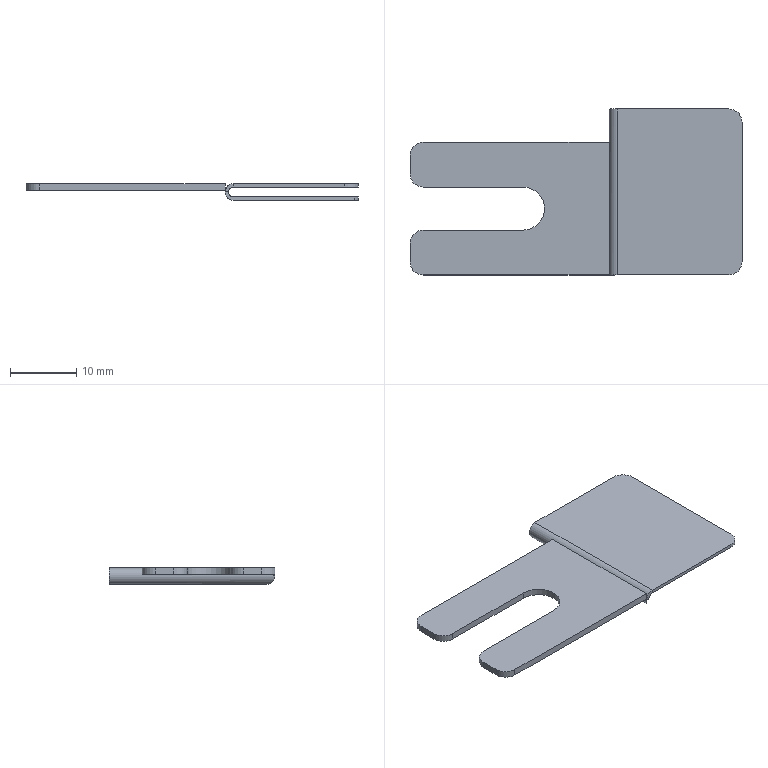Part | SolidWorks | features ICE 4, Fillet 2, FlatPattern 2, SMBaseFlange 2, SheetMetal 2, MirrorSolid 1 | 2 solids | 33 faces | box 50 x 25 x 2.5 mm | volume 876.083 mm3 | plane 22 | cylinder 11 | commonest cylinder face diameters 4 x8 1.5 x1 2.5 x1 6.5 x1
STEP:
#1=CARTESIAN_POINT('',(1.25,0.,0.));
#2=VERTEX_POINT('',#1);
#3=CARTESIAN_POINT('',(0.,0.,-1.25));
#4=VERTEX_POINT('',#3);
#5=CARTESIAN_POINT('',(1.25,0.,-1.25));
#6=DIRECTION('',(0.,-1.,0.));
#7=DIRECTION('',(0.,0.,1.));
#8=AXIS2_PLACEMENT_3D('',#5,#6,#7);
#9=CIRCLE('',#8,1.25);
#10=EDGE_CURVE('',#2,#4,#9,.T.);
#11=ORIENTED_EDGE('',*,*,#10,.T.);
#12=CARTESIAN_POINT('',(0.5,0.,-1.25));
#13=VERTEX_POINT('',#12);
#14=CARTESIAN_POINT('',(20.,0.,-1.25));
#15=DIRECTION('',(-1.,0.,0.));
#16=VECTOR('',#15,1000.);
#17=LINE('',#14,#16);
#18=EDGE_CURVE('',#13,#4,#17,.T.);
#19=ORIENTED_EDGE('',*,*,#18,.F.);
#20=CARTESIAN_POINT('',(1.25,0.,-0.5));
#21=VERTEX_POINT('',#20);
#22=CARTESIAN_POINT('',(1.25,0.,-1.25));
#23=DIRECTION('',(0.,-1.,0.));
#24=DIRECTION('',(1.,0.,0.));
#25=AXIS2_PLACEMENT_3D('',#22,#23,#24);
#26=CIRCLE('',#25,0.75);
#27=EDGE_CURVE('',#21,#13,#26,.T.);
#28=ORIENTED_EDGE('',*,*,#27,.F.);
#29=CARTESIAN_POINT('',(1.25,0.,0.));
#30=DIRECTION('',(0.,0.,-1.));
#31=VECTOR('',#30,1000.);
#32=LINE('',#29,#31);
#33=EDGE_CURVE('',#2,#21,#32,.T.);
#34=ORIENTED_EDGE('',*,*,#33,.F.);
#35=EDGE_LOOP('',(#11,#19,#28,#34));
#36=FACE_OUTER_BOUND('',#35,.T.);
#37=CARTESIAN_POINT('',(1.25,0.,0.));
#38=DIRECTION('',(0.,-1.,0.));
#39=DIRECTION('',(0.,0.,-1.));
#40=AXIS2_PLACEMENT_3D('',#37,#38,#39);
#41=PLANE('',#40);
#42=ADVANCED_FACE('',(#36),#41,.T.);
#43=CARTESIAN_POINT('',(1.25,25.,-2.5));
#44=VERTEX_POINT('',#43);
#45=CARTESIAN_POINT('',(1.25,25.,-2.));
#46=VERTEX_POINT('',#45);
#47=CARTESIAN_POINT('',(1.25,25.,-2.5));
#48=DIRECTION('',(0.,0.,1.));
#49=VECTOR('',#48,1000.);
#50=LINE('',#47,#49);
#51=EDGE_CURVE('',#44,#46,#50,.T.);
#52=ORIENTED_EDGE('',*,*,#51,.F.);
#53=CARTESIAN_POINT('',(1.25,25.,0.));
#54=VERTEX_POINT('',#53);
#55=CARTESIAN_POINT('',(1.25,25.,-1.25));
#56=DIRECTION('',(0.,-1.,0.));
#57=DIRECTION('',(0.,0.,1.));
#58=AXIS2_PLACEMENT_3D('',#55,#56,#57);
#59=CIRCLE('',#58,1.25);
#60=EDGE_CURVE('',#54,#44,#59,.T.);
#61=ORIENTED_EDGE('',*,*,#60,.F.);
#62=CARTESIAN_POINT('',(1.25,25.,-0.5));
#63=VERTEX_POINT('',#62);
#64=CARTESIAN_POINT('',(1.25,25.,-0.5));
#65=DIRECTION('',(0.,0.,1.));
#66=VECTOR('',#65,1000.);
#67=LINE('',#64,#66);
#68=EDGE_CURVE('',#63,#54,#67,.T.);
#69=ORIENTED_EDGE('',*,*,#68,.F.);
#70=CARTESIAN_POINT('',(1.25,25.,-1.25));
#71=DIRECTION('',(0.,-1.,0.));
#72=DIRECTION('',(1.,0.,0.));
#73=AXIS2_PLACEMENT_3D('',#70,#71,#72);
#74=CIRCLE('',#73,0.75);
#75=EDGE_CURVE('',#63,#46,#74,.T.);
#76=ORIENTED_EDGE('',*,*,#75,.T.);
#77=EDGE_LOOP('',(#52,#61,#69,#76));
#78=FACE_OUTER_BOUND('',#77,.T.);
#79=CARTESIAN_POINT('',(1.25,25.,-2.5));
#80=DIRECTION('',(0.,1.,0.));
#81=DIRECTION('',(0.,0.,1.));
#82=AXIS2_PLACEMENT_3D('',#79,#80,#81);
#83=PLANE('',#82);
#84=ADVANCED_FACE('',(#78),#83,.T.);
#85=CARTESIAN_POINT('',(18.,25.,-2.));
#86=VERTEX_POINT('',#85);
#87=CARTESIAN_POINT('',(1.25,25.,-2.));
#88=DIRECTION('',(1.,0.,0.));
#89=VECTOR('',#88,1000.);
#90=LINE('',#87,#89);
#91=EDGE_CURVE('',#46,#86,#90,.T.);
#92=ORIENTED_EDGE('',*,*,#91,.T.);
#93=CARTESIAN_POINT('',(18.,25.,-2.5));
#94=VERTEX_POINT('',#93);
#95=CARTESIAN_POINT('',(18.,25.,-0.5));
#96=DIRECTION('',(0.,0.,-1.));
#97=VECTOR('',#96,1000.);
#98=LINE('',#95,#97);
#99=EDGE_CURVE('',#86,#94,#98,.T.);
#100=ORIENTED_EDGE('',*,*,#99,.T.);
#101=CARTESIAN_POINT('',(1.25,25.,-2.5));
#102=DIRECTION('',(1.,0.,0.));
#103=VECTOR('',#102,1000.);
#104=LINE('',#101,#103);
#105=EDGE_CURVE('',#44,#94,#104,.T.);
#106=ORIENTED_EDGE('',*,*,#105,.F.);
#107=ORIENTED_EDGE('',*,*,#51,.T.);
#108=EDGE_LOOP('',(#92,#100,#106,#107));
#109=FACE_OUTER_BOUND('',#108,.T.);
#110=CARTESIAN_POINT('',(1.25,25.,-0.5));
#111=DIRECTION('',(0.,1.,0.));
#112=DIRECTION('',(0.,0.,1.));
#113=AXIS2_PLACEMENT_3D('',#110,#111,#112);
#114=PLANE('',#113);
#115=ADVANCED_FACE('',(#109),#114,.T.);
#116=CARTESIAN_POINT('',(18.,0.,-0.5));
#117=VERTEX_POINT('',#116);
#118=CARTESIAN_POINT('',(20.,0.,-0.5));
#119=DIRECTION('',(-1.,0.,0.));
#120=VECTOR('',#119,1000.);
#121=LINE('',#118,#120);
#122=EDGE_CURVE('',#117,#21,#121,.T.);
#123=ORIENTED_EDGE('',*,*,#122,.F.);
#124=CARTESIAN_POINT('',(18.,0.,0.));
#125=VERTEX_POINT('',#124);
#126=CARTESIAN_POINT('',(18.,0.,-2.));
#127=DIRECTION('',(0.,0.,1.));
#128=VECTOR('',#127,1000.);
#129=LINE('',#126,#128);
#130=EDGE_CURVE('',#117,#125,#129,.T.);
#131=ORIENTED_EDGE('',*,*,#130,.T.);
#132=CARTESIAN_POINT('',(20.,0.,0.));
#133=DIRECTION('',(-1.,0.,0.));
#134=VECTOR('',#133,1000.);
#135=LINE('',#132,#134);
#136=EDGE_CURVE('',#125,#2,#135,.T.);
#137=ORIENTED_EDGE('',*,*,#136,.T.);
#138=ORIENTED_EDGE('',*,*,#33,.T.);
#139=EDGE_LOOP('',(#123,#131,#137,#138));
#140=FACE_OUTER_BOUND('',#139,.T.);
#141=CARTESIAN_POINT('',(1.25,0.,-2.));
#142=DIRECTION('',(0.,-1.,0.));
#143=DIRECTION('',(0.,0.,-1.));
#144=AXIS2_PLACEMENT_3D('',#141,#142,#143);
#145=PLANE('',#144);
#146=ADVANCED_FACE('',(#140),#145,.T.);
#147=CARTESIAN_POINT('',(20.,23.,-2.));
#148=VERTEX_POINT('',#147);
#149=CARTESIAN_POINT('',(20.,20.828,-2.));
#150=VERTEX_POINT('',#149);
#151=CARTESIAN_POINT('',(20.,25.,-2.));
#152=DIRECTION('',(0.,-1.,0.));
#153=VECTOR('',#152,1000.);
#154=LINE('',#151,#153);
#155=EDGE_CURVE('',#148,#150,#154,.T.);
#156=ORIENTED_EDGE('',*,*,#155,.F.);
#157=CARTESIAN_POINT('',(18.,23.,-2.));
#158=DIRECTION('',(0.,0.,1.));
#159=DIRECTION('',(-1.,0.,0.));
#160=AXIS2_PLACEMENT_3D('',#157,#158,#159);
#161=CIRCLE('',#160,2.);
#162=EDGE_CURVE('',#148,#86,#161,.T.);
#163=ORIENTED_EDGE('',*,*,#162,.T.);
#164=ORIENTED_EDGE('',*,*,#91,.F.);
#165=CARTESIAN_POINT('',(1.25,1.25,-2.));
#166=VERTEX_POINT('',#165);
#167=CARTESIAN_POINT('',(1.25,25.,-2.));
#168=DIRECTION('',(0.,-1.,0.));
#169=VECTOR('',#168,1000.);
#170=LINE('',#167,#169);
#171=EDGE_CURVE('',#46,#166,#170,.T.);
#172=ORIENTED_EDGE('',*,*,#171,.T.);
#173=CARTESIAN_POINT('',(19.414,19.414,-2.));
#174=VERTEX_POINT('',#173);
#175=CARTESIAN_POINT('',(13.125,13.125,-2.));
#176=DIRECTION('',(0.7071,0.7071,0.));
#177=VECTOR('',#176,1000.);
#178=LINE('',#175,#177);
#179=EDGE_CURVE('',#166,#174,#178,.T.);
#180=ORIENTED_EDGE('',*,*,#179,.T.);
#181=CARTESIAN_POINT('',(18.,20.828,-2.));
#182=DIRECTION('',(0.,0.,1.));
#183=DIRECTION('',(-1.,0.,0.));
#184=AXIS2_PLACEMENT_3D('',#181,#182,#183);
#185=CIRCLE('',#184,2.);
#186=EDGE_CURVE('',#174,#150,#185,.T.);
#187=ORIENTED_EDGE('',*,*,#186,.T.);
#188=EDGE_LOOP('',(#156,#163,#164,#172,#180,#187));
#189=FACE_OUTER_BOUND('',#188,.T.);
#190=CARTESIAN_POINT('',(1.25,25.,-2.));
#191=DIRECTION('',(0.,0.,-1.));
#192=DIRECTION('',(-1.,0.,0.));
#193=AXIS2_PLACEMENT_3D('',#190,#191,#192);
#194=PLANE('',#193);
#195=ADVANCED_FACE('',(#189),#194,.F.);
#196=CARTESIAN_POINT('',(20.,23.,-2.5));
#197=VERTEX_POINT('',#196);
#198=CARTESIAN_POINT('',(20.,20.828,-2.5));
#199=VERTEX_POINT('',#198);
#200=CARTESIAN_POINT('',(20.,25.,-2.5));
#201=DIRECTION('',(0.,-1.,0.));
#202=VECTOR('',#201,1000.);
#203=LINE('',#200,#202);
#204=EDGE_CURVE('',#197,#199,#203,.T.);
#205=ORIENTED_EDGE('',*,*,#204,.F.);
#206=CARTESIAN_POINT('',(20.,23.,-2.5));
#207=DIRECTION('',(0.,0.,1.));
#208=VECTOR('',#207,1000.);
#209=LINE('',#206,#208);
#210=EDGE_CURVE('',#197,#148,#209,.T.);
#211=ORIENTED_EDGE('',*,*,#210,.T.);
#212=ORIENTED_EDGE('',*,*,#155,.T.);
#213=CARTESIAN_POINT('',(20.,20.828,-2.5));
#214=DIRECTION('',(0.,0.,-1.));
#215=VECTOR('',#214,1000.);
#216=LINE('',#213,#215);
#217=EDGE_CURVE('',#150,#199,#216,.T.);
#218=ORIENTED_EDGE('',*,*,#217,.T.);
#219=EDGE_LOOP('',(#205,#211,#212,#218));
#220=FACE_OUTER_BOUND('',#219,.T.);
#221=CARTESIAN_POINT('',(20.,25.,-2.5));
#222=DIRECTION('',(1.,0.,0.));
#223=DIRECTION('',(0.,0.,-1.));
#224=AXIS2_PLACEMENT_3D('',#221,#222,#223);
#225=PLANE('',#224);
#226=ADVANCED_FACE('',(#220),#225,.T.);
#227=ORIENTED_EDGE('',*,*,#105,.T.);
#228=CARTESIAN_POINT('',(18.,23.,-2.5));
#229=DIRECTION('',(0.,0.,-1.));
#230=DIRECTION('',(-1.,0.,0.));
#231=AXIS2_PLACEMENT_3D('',#228,#229,#230);
#232=CIRCLE('',#231,2.);
#233=EDGE_CURVE('',#94,#197,#232,.T.);
#234=ORIENTED_EDGE('',*,*,#233,.T.);
#235=ORIENTED_EDGE('',*,*,#204,.T.);
#236=CARTESIAN_POINT('',(19.414,19.414,-2.5));
#237=VERTEX_POINT('',#236);
#238=CARTESIAN_POINT('',(18.,20.828,-2.5));
#239=DIRECTION('',(0.,0.,-1.));
#240=DIRECTION('',(-1.,0.,0.));
#241=AXIS2_PLACEMENT_3D('',#238,#239,#240);
#242=CIRCLE('',#241,2.);
#243=EDGE_CURVE('',#199,#237,#242,.T.);
#244=ORIENTED_EDGE('',*,*,#243,.T.);
#245=CARTESIAN_POINT('',(1.25,1.25,-2.5));
#246=VERTEX_POINT('',#245);
#247=CARTESIAN_POINT('',(0.,0.,-2.5));
#248=DIRECTION('',(0.7071,0.7071,0.));
#249=VECTOR('',#248,1000.);
#250=LINE('',#247,#249);
#251=EDGE_CURVE('',#246,#237,#250,.T.);
#252=ORIENTED_EDGE('',*,*,#251,.F.);
#253=CARTESIAN_POINT('',(1.25,25.,-2.5));
#254=DIRECTION('',(0.,-1.,0.));
#255=VECTOR('',#254,1000.);
#256=LINE('',#253,#255);
#257=EDGE_CURVE('',#44,#246,#256,.T.);
#258=ORIENTED_EDGE('',*,*,#257,.F.);
#259=EDGE_LOOP('',(#227,#234,#235,#244,#252,#258));
#260=FACE_OUTER_BOUND('',#259,.T.);
#261=CARTESIAN_POINT('',(1.25,25.,-2.5));
#262=DIRECTION('',(0.,0.,-1.));
#263=DIRECTION('',(-1.,0.,0.));
#264=AXIS2_PLACEMENT_3D('',#261,#262,#263);
#265=PLANE('',#264);
#266=ADVANCED_FACE('',(#260),#265,.T.);
#267=CARTESIAN_POINT('',(0.,0.,-1.25));
#268=CARTESIAN_POINT('',(0.,0.,-1.982));
#269=CARTESIAN_POINT('',(0.5178,0.5178,-2.5));
#270=CARTESIAN_POINT('',(1.25,1.25,-2.5));
#271=(BOUNDED_CURVE()B_SPLINE_CURVE(3,(#267,#268,#269,#270),.UNSPECIFIED.,.F.,.F.)B_SPLINE_CURVE_WITH_KNOTS((4,4),(0.,1.571),.UNSPECIFIED.)CURVE()GEOMETRIC_REPRESENTATION_ITEM()RATIONAL_B_SPLINE_CURVE((1.,0.8047,0.8047,1.))REPRESENTATION_ITEM(''));
#272=EDGE_CURVE('',#4,#246,#271,.T.);
#273=ORIENTED_EDGE('',*,*,#272,.F.);
#274=ORIENTED_EDGE('',*,*,#10,.F.);
#275=CARTESIAN_POINT('',(1.25,25.,0.));
#276=DIRECTION('',(0.,-1.,0.));
#277=VECTOR('',#276,1000.);
#278=LINE('',#275,#277);
#279=EDGE_CURVE('',#54,#2,#278,.T.);
#280=ORIENTED_EDGE('',*,*,#279,.F.);
#281=ORIENTED_EDGE('',*,*,#60,.T.);
#282=ORIENTED_EDGE('',*,*,#257,.T.);
#283=EDGE_LOOP('',(#273,#274,#280,#281,#282));
#284=FACE_OUTER_BOUND('',#283,.T.);
#285=CARTESIAN_POINT('',(1.25,25.,-1.25));
#286=DIRECTION('',(0.,-1.,0.));
#287=DIRECTION('',(0.,0.,-1.));
#288=AXIS2_PLACEMENT_3D('',#285,#286,#287);
#289=CYLINDRICAL_SURFACE('',#288,1.25);
#290=ADVANCED_FACE('',(#284),#289,.T.);
#291=ORIENTED_EDGE('',*,*,#136,.F.);
#292=CARTESIAN_POINT('',(20.,2.,0.));
#293=VERTEX_POINT('',#292);
#294=CARTESIAN_POINT('',(18.,2.,0.));
#295=DIRECTION('',(0.,0.,1.));
#296=DIRECTION('',(1.,0.,0.));
#297=AXIS2_PLACEMENT_3D('',#294,#295,#296);
#298=CIRCLE('',#297,2.);
#299=EDGE_CURVE('',#125,#293,#298,.T.);
#300=ORIENTED_EDGE('',*,*,#299,.T.);
#301=CARTESIAN_POINT('',(20.,23.,0.));
#302=VERTEX_POINT('',#301);
#303=CARTESIAN_POINT('',(20.,25.,0.));
#304=DIRECTION('',(0.,-1.,0.));
#305=VECTOR('',#304,1000.);
#306=LINE('',#303,#305);
#307=EDGE_CURVE('',#302,#293,#306,.T.);
#308=ORIENTED_EDGE('',*,*,#307,.F.);
#309=CARTESIAN_POINT('',(18.,25.,0.));
#310=VERTEX_POINT('',#309);
#311=CARTESIAN_POINT('',(18.,23.,0.));
#312=DIRECTION('',(0.,0.,1.));
#313=DIRECTION('',(1.,0.,0.));
#314=AXIS2_PLACEMENT_3D('',#311,#312,#313);
#315=CIRCLE('',#314,2.);
#316=EDGE_CURVE('',#302,#310,#315,.T.);
#317=ORIENTED_EDGE('',*,*,#316,.T.);
#318=CARTESIAN_POINT('',(20.,25.,0.));
#319=DIRECTION('',(-1.,0.,0.));
#320=VECTOR('',#319,1000.);
#321=LINE('',#318,#320);
#322=EDGE_CURVE('',#310,#54,#321,.T.);
#323=ORIENTED_EDGE('',*,*,#322,.T.);
#324=ORIENTED_EDGE('',*,*,#279,.T.);
#325=EDGE_LOOP('',(#291,#300,#308,#317,#323,#324));
#326=FACE_OUTER_BOUND('',#325,.T.);
#327=CARTESIAN_POINT('',(20.,25.,0.));
#328=DIRECTION('',(0.,0.,1.));
#329=DIRECTION('',(1.,0.,0.));
#330=AXIS2_PLACEMENT_3D('',#327,#328,#329);
#331=PLANE('',#330);
#332=ADVANCED_FACE('',(#326),#331,.T.);
#333=ORIENTED_EDGE('',*,*,#307,.T.);
#334=CARTESIAN_POINT('',(20.,2.,-0.5));
#335=VERTEX_POINT('',#334);
#336=CARTESIAN_POINT('',(20.,2.,-0.5));
#337=DIRECTION('',(0.,0.,-1.));
#338=VECTOR('',#337,1000.);
#339=LINE('',#336,#338);
#340=EDGE_CURVE('',#293,#335,#339,.T.);
#341=ORIENTED_EDGE('',*,*,#340,.T.);
#342=CARTESIAN_POINT('',(20.,23.,-0.5));
#343=VERTEX_POINT('',#342);
#344=CARTESIAN_POINT('',(20.,25.,-0.5));
#345=DIRECTION('',(0.,-1.,0.));
#346=VECTOR('',#345,1000.);
#347=LINE('',#344,#346);
#348=EDGE_CURVE('',#343,#335,#347,.T.);
#349=ORIENTED_EDGE('',*,*,#348,.F.);
#350=CARTESIAN_POINT('',(20.,23.,0.));
#351=DIRECTION('',(0.,0.,1.));
#352=VECTOR('',#351,1000.);
#353=LINE('',#350,#352);
#354=EDGE_CURVE('',#343,#302,#353,.T.);
#355=ORIENTED_EDGE('',*,*,#354,.T.);
#356=EDGE_LOOP('',(#333,#341,#349,#355));
#357=FACE_OUTER_BOUND('',#356,.T.);
#358=CARTESIAN_POINT('',(20.,25.,-0.5));
#359=DIRECTION('',(1.,0.,0.));
#360=DIRECTION('',(0.,0.,-1.));
#361=AXIS2_PLACEMENT_3D('',#358,#359,#360);
#362=PLANE('',#361);
#363=ADVANCED_FACE('',(#357),#362,.T.);
#364=ORIENTED_EDGE('',*,*,#348,.T.);
#365=CARTESIAN_POINT('',(18.,2.,-0.5));
#366=DIRECTION('',(0.,0.,-1.));
#367=DIRECTION('',(1.,0.,0.));
#368=AXIS2_PLACEMENT_3D('',#365,#366,#367);
#369=CIRCLE('',#368,2.);
#370=EDGE_CURVE('',#335,#117,#369,.T.);
#371=ORIENTED_EDGE('',*,*,#370,.T.);
#372=ORIENTED_EDGE('',*,*,#122,.T.);
#373=CARTESIAN_POINT('',(1.25,25.,-0.5));
#374=DIRECTION('',(0.,-1.,0.));
#375=VECTOR('',#374,1000.);
#376=LINE('',#373,#375);
#377=EDGE_CURVE('',#63,#21,#376,.T.);
#378=ORIENTED_EDGE('',*,*,#377,.F.);
#379=CARTESIAN_POINT('',(18.,25.,-0.5));
#380=VERTEX_POINT('',#379);
#381=CARTESIAN_POINT('',(20.,25.,-0.5));
#382=DIRECTION('',(-1.,0.,0.));
#383=VECTOR('',#382,1000.);
#384=LINE('',#381,#383);
#385=EDGE_CURVE('',#380,#63,#384,.T.);
#386=ORIENTED_EDGE('',*,*,#385,.F.);
#387=CARTESIAN_POINT('',(18.,23.,-0.5));
#388=DIRECTION('',(0.,0.,-1.));
#389=DIRECTION('',(1.,0.,0.));
#390=AXIS2_PLACEMENT_3D('',#387,#388,#389);
#391=CIRCLE('',#390,2.);
#392=EDGE_CURVE('',#380,#343,#391,.T.);
#393=ORIENTED_EDGE('',*,*,#392,.T.);
#394=EDGE_LOOP('',(#364,#371,#372,#378,#386,#393));
#395=FACE_OUTER_BOUND('',#394,.T.);
#396=CARTESIAN_POINT('',(20.,25.,-0.5));
#397=DIRECTION('',(0.,0.,1.));
#398=DIRECTION('',(1.,0.,0.));
#399=AXIS2_PLACEMENT_3D('',#396,#397,#398);
#400=PLANE('',#399);
#401=ADVANCED_FACE('',(#395),#400,.F.);
#402=CARTESIAN_POINT('',(0.5,0.5,-1.25));
#403=VERTEX_POINT('',#402);
#404=CARTESIAN_POINT('',(0.5,25.,-1.25));
#405=DIRECTION('',(0.,-1.,0.));
#406=VECTOR('',#405,1000.);
#407=LINE('',#404,#406);
#408=EDGE_CURVE('',#403,#13,#407,.T.);
#409=ORIENTED_EDGE('',*,*,#408,.F.);
#410=CARTESIAN_POINT('',(0.5,0.5,-1.25));
#411=CARTESIAN_POINT('',(0.5,0.5,-1.689));
#412=CARTESIAN_POINT('',(0.8107,0.8107,-2.));
#413=CARTESIAN_POINT('',(1.25,1.25,-2.));
#414=(BOUNDED_CURVE()B_SPLINE_CURVE(3,(#410,#411,#412,#413),.UNSPECIFIED.,.F.,.F.)B_SPLINE_CURVE_WITH_KNOTS((4,4),(0.,1.571),.UNSPECIFIED.)CURVE()GEOMETRIC_REPRESENTATION_ITEM()RATIONAL_B_SPLINE_CURVE((1.,0.8047,0.8047,1.))REPRESENTATION_ITEM(''));
#415=EDGE_CURVE('',#403,#166,#414,.T.);
#416=ORIENTED_EDGE('',*,*,#415,.T.);
#417=ORIENTED_EDGE('',*,*,#171,.F.);
#418=ORIENTED_EDGE('',*,*,#75,.F.);
#419=ORIENTED_EDGE('',*,*,#377,.T.);
#420=ORIENTED_EDGE('',*,*,#27,.T.);
#421=EDGE_LOOP('',(#409,#416,#417,#418,#419,#420));
#422=FACE_OUTER_BOUND('',#421,.T.);
#423=CARTESIAN_POINT('',(1.25,25.,-1.25));
#424=DIRECTION('',(0.,-1.,0.));
#425=DIRECTION('',(0.,0.,-1.));
#426=AXIS2_PLACEMENT_3D('',#423,#424,#425);
#427=CYLINDRICAL_SURFACE('',#426,0.75);
#428=ADVANCED_FACE('',(#422),#427,.F.);
#429=ORIENTED_EDGE('',*,*,#322,.F.);
#430=CARTESIAN_POINT('',(18.,25.,-0.5));
#431=DIRECTION('',(0.,0.,-1.));
#432=VECTOR('',#431,1000.);
#433=LINE('',#430,#432);
#434=EDGE_CURVE('',#310,#380,#433,.T.);
#435=ORIENTED_EDGE('',*,*,#434,.T.);
#436=ORIENTED_EDGE('',*,*,#385,.T.);
#437=ORIENTED_EDGE('',*,*,#68,.T.);
#438=EDGE_LOOP('',(#429,#435,#436,#437));
#439=FACE_OUTER_BOUND('',#438,.T.);
#440=CARTESIAN_POINT('',(1.25,25.,-1.25));
#441=DIRECTION('',(0.,-1.,0.));
#442=DIRECTION('',(-1.,0.,0.));
#443=AXIS2_PLACEMENT_3D('',#440,#441,#442);
#444=PLANE('',#443);
#445=ADVANCED_FACE('',(#439),#444,.F.);
#446=ORIENTED_EDGE('',*,*,#251,.T.);
#447=CARTESIAN_POINT('',(19.414,19.414,-2.));
#448=DIRECTION('',(0.,0.,1.));
#449=VECTOR('',#448,1000.);
#450=LINE('',#447,#449);
#451=EDGE_CURVE('',#237,#174,#450,.T.);
#452=ORIENTED_EDGE('',*,*,#451,.T.);
#453=ORIENTED_EDGE('',*,*,#179,.F.);
#454=ORIENTED_EDGE('',*,*,#415,.F.);
#455=CARTESIAN_POINT('',(0.,0.,-1.25));
#456=DIRECTION('',(0.7071,0.7071,0.));
#457=VECTOR('',#456,1000.);
#458=LINE('',#455,#457);
#459=EDGE_CURVE('',#4,#403,#458,.T.);
#460=ORIENTED_EDGE('',*,*,#459,.F.);
#461=ORIENTED_EDGE('',*,*,#272,.T.);
#462=EDGE_LOOP('',(#446,#452,#453,#454,#460,#461));
#463=FACE_OUTER_BOUND('',#462,.T.);
#464=CARTESIAN_POINT('',(0.,0.,-1.25));
#465=DIRECTION('',(-0.7071,0.7071,0.));
#466=DIRECTION('',(-0.7071,-0.7071,0.));
#467=AXIS2_PLACEMENT_3D('',#464,#465,#466);
#468=PLANE('',#467);
#469=ADVANCED_FACE('',(#463),#468,.F.);
#470=ORIENTED_EDGE('',*,*,#408,.T.);
#471=ORIENTED_EDGE('',*,*,#18,.T.);
#472=ORIENTED_EDGE('',*,*,#459,.T.);
#473=EDGE_LOOP('',(#470,#471,#472));
#474=FACE_OUTER_BOUND('',#473,.T.);
#475=CARTESIAN_POINT('',(0.,0.,-1.25));
#476=DIRECTION('',(0.,0.,-1.));
#477=DIRECTION('',(-1.,0.,0.));
#478=AXIS2_PLACEMENT_3D('',#475,#476,#477);
#479=PLANE('',#478);
#480=ADVANCED_FACE('',(#474),#479,.T.);
#481=ORIENTED_EDGE('',*,*,#370,.F.);
#482=ORIENTED_EDGE('',*,*,#340,.F.);
#483=ORIENTED_EDGE('',*,*,#299,.F.);
#484=ORIENTED_EDGE('',*,*,#130,.F.);
#485=EDGE_LOOP('',(#481,#482,#483,#484));
#486=FACE_OUTER_BOUND('',#485,.T.);
#487=CARTESIAN_POINT('',(18.,2.,-2.));
#488=DIRECTION('',(0.,0.,1.));
#489=DIRECTION('',(1.,0.,0.));
#490=AXIS2_PLACEMENT_3D('',#487,#488,#489);
#491=CYLINDRICAL_SURFACE('',#490,2.);
#492=ADVANCED_FACE('',(#486),#491,.T.);
#493=ORIENTED_EDGE('',*,*,#392,.F.);
#494=ORIENTED_EDGE('',*,*,#434,.F.);
#495=ORIENTED_EDGE('',*,*,#316,.F.);
#496=ORIENTED_EDGE('',*,*,#354,.F.);
#497=EDGE_LOOP('',(#493,#494,#495,#496));
#498=FACE_OUTER_BOUND('',#497,.T.);
#499=CARTESIAN_POINT('',(18.,23.,-0.5));
#500=DIRECTION('',(0.,0.,-1.));
#501=DIRECTION('',(-1.,0.,0.));
#502=AXIS2_PLACEMENT_3D('',#499,#500,#501);
#503=CYLINDRICAL_SURFACE('',#502,2.);
#504=ADVANCED_FACE('',(#498),#503,.T.);
#505=ORIENTED_EDGE('',*,*,#233,.F.);
#506=ORIENTED_EDGE('',*,*,#99,.F.);
#507=ORIENTED_EDGE('',*,*,#162,.F.);
#508=ORIENTED_EDGE('',*,*,#210,.F.);
#509=EDGE_LOOP('',(#505,#506,#507,#508));
#510=FACE_OUTER_BOUND('',#509,.T.);
#511=CARTESIAN_POINT('',(18.,23.,-2.5));
#512=DIRECTION('',(0.,0.,1.));
#513=DIRECTION('',(1.,0.,0.));
#514=AXIS2_PLACEMENT_3D('',#511,#512,#513);
#515=CYLINDRICAL_SURFACE('',#514,2.);
#516=ADVANCED_FACE('',(#510),#515,.T.);
#517=ORIENTED_EDGE('',*,*,#186,.F.);
#518=ORIENTED_EDGE('',*,*,#451,.F.);
#519=ORIENTED_EDGE('',*,*,#243,.F.);
#520=ORIENTED_EDGE('',*,*,#217,.F.);
#521=EDGE_LOOP('',(#517,#518,#519,#520));
#522=FACE_OUTER_BOUND('',#521,.T.);
#523=CARTESIAN_POINT('',(18.,20.828,-2.5));
#524=DIRECTION('',(0.,0.,1.));
#525=DIRECTION('',(1.,0.,0.));
#526=AXIS2_PLACEMENT_3D('',#523,#524,#525);
#527=CYLINDRICAL_SURFACE('',#526,2.);
#528=ADVANCED_FACE('',(#522),#527,.T.);
#529=CLOSED_SHELL('',(#42,#84,#115,#146,#195,#226,#266,#290,#332,#363,#401,#428,#445,#469,#480,#492,#504,#516,#528));
#530=MANIFOLD_SOLID_BREP('',#529);
#531=CARTESIAN_POINT('',(-30.,4.75,0.));
#532=VERTEX_POINT('',#531);
#533=CARTESIAN_POINT('',(-30.,2.,0.));
#534=VERTEX_POINT('',#533);
#535=CARTESIAN_POINT('',(-30.,20.,0.));
#536=DIRECTION('',(0.,-1.,0.));
#537=VECTOR('',#536,1000.);
#538=LINE('',#535,#537);
#539=EDGE_CURVE('',#532,#534,#538,.T.);
#540=ORIENTED_EDGE('',*,*,#539,.F.);
#541=CARTESIAN_POINT('',(-30.,4.75,-1.));
#542=VERTEX_POINT('',#541);
#543=CARTESIAN_POINT('',(-30.,4.75,-1.));
#544=DIRECTION('',(0.,0.,-1.));
#545=VECTOR('',#544,1000.);
#546=LINE('',#543,#545);
#547=EDGE_CURVE('',#532,#542,#546,.T.);
#548=ORIENTED_EDGE('',*,*,#547,.T.);
#549=CARTESIAN_POINT('',(-30.,2.,-1.));
#550=VERTEX_POINT('',#549);
#551=CARTESIAN_POINT('',(-30.,20.,-1.));
#552=DIRECTION('',(0.,-1.,0.));
#553=VECTOR('',#552,1000.);
#554=LINE('',#551,#553);
#555=EDGE_CURVE('',#542,#550,#554,.T.);
#556=ORIENTED_EDGE('',*,*,#555,.T.);
#557=CARTESIAN_POINT('',(-30.,2.,0.));
#558=DIRECTION('',(0.,0.,1.));
#559=VECTOR('',#558,1000.);
#560=LINE('',#557,#559);
#561=EDGE_CURVE('',#550,#534,#560,.T.);
#562=ORIENTED_EDGE('',*,*,#561,.T.);
#563=EDGE_LOOP('',(#540,#548,#556,#562));
#564=FACE_OUTER_BOUND('',#563,.T.);
#565=CARTESIAN_POINT('',(-30.,20.,0.));
#566=DIRECTION('',(-1.,0.,0.));
#567=DIRECTION('',(0.,0.,1.));
#568=AXIS2_PLACEMENT_3D('',#565,#566,#567);
#569=PLANE('',#568);
#570=ADVANCED_FACE('',(#564),#569,.T.);
#571=CARTESIAN_POINT('',(-30.,18.,-1.));
#572=VERTEX_POINT('',#571);
#573=CARTESIAN_POINT('',(-30.,15.25,-1.));
#574=VERTEX_POINT('',#573);
#575=CARTESIAN_POINT('',(-30.,20.,-1.));
#576=DIRECTION('',(0.,-1.,0.));
#577=VECTOR('',#576,1000.);
#578=LINE('',#575,#577);
#579=EDGE_CURVE('',#572,#574,#578,.T.);
#580=ORIENTED_EDGE('',*,*,#579,.F.);
#581=CARTESIAN_POINT('',(-28.,20.,-1.));
#582=VERTEX_POINT('',#581);
#583=CARTESIAN_POINT('',(-28.,18.,-1.));
#584=DIRECTION('',(0.,0.,-1.));
#585=DIRECTION('',(1.,0.,0.));
#586=AXIS2_PLACEMENT_3D('',#583,#584,#585);
#587=CIRCLE('',#586,2.);
#588=EDGE_CURVE('',#572,#582,#587,.T.);
#589=ORIENTED_EDGE('',*,*,#588,.T.);
#590=CARTESIAN_POINT('',(0.,20.,-1.));
#591=VERTEX_POINT('',#590);
#592=CARTESIAN_POINT('',(0.,20.,-1.));
#593=DIRECTION('',(-1.,0.,0.));
#594=VECTOR('',#593,1000.);
#595=LINE('',#592,#594);
#596=EDGE_CURVE('',#591,#582,#595,.T.);
#597=ORIENTED_EDGE('',*,*,#596,.F.);
#598=CARTESIAN_POINT('',(0.,0.,-1.));
#599=VERTEX_POINT('',#598);
#600=CARTESIAN_POINT('',(0.,20.,-1.));
#601=DIRECTION('',(0.,-1.,0.));
#602=VECTOR('',#601,1000.);
#603=LINE('',#600,#602);
#604=EDGE_CURVE('',#591,#599,#603,.T.);
#605=ORIENTED_EDGE('',*,*,#604,.T.);
#606=CARTESIAN_POINT('',(-28.,0.,-1.));
#607=VERTEX_POINT('',#606);
#608=CARTESIAN_POINT('',(0.,0.,-1.));
#609=DIRECTION('',(-1.,0.,0.));
#610=VECTOR('',#609,1000.);
#611=LINE('',#608,#610);
#612=EDGE_CURVE('',#599,#607,#611,.T.);
#613=ORIENTED_EDGE('',*,*,#612,.T.);
#614=CARTESIAN_POINT('',(-28.,2.,-1.));
#615=DIRECTION('',(0.,0.,-1.));
#616=DIRECTION('',(1.,0.,0.));
#617=AXIS2_PLACEMENT_3D('',#614,#615,#616);
#618=CIRCLE('',#617,2.);
#619=EDGE_CURVE('',#607,#550,#618,.T.);
#620=ORIENTED_EDGE('',*,*,#619,.T.);
#621=ORIENTED_EDGE('',*,*,#555,.F.);
#622=CARTESIAN_POINT('',(-28.,6.75,-1.));
#623=VERTEX_POINT('',#622);
#624=CARTESIAN_POINT('',(-28.,4.75,-1.));
#625=DIRECTION('',(0.,0.,-1.));
#626=DIRECTION('',(1.,0.,0.));
#627=AXIS2_PLACEMENT_3D('',#624,#625,#626);
#628=CIRCLE('',#627,2.);
#629=EDGE_CURVE('',#542,#623,#628,.T.);
#630=ORIENTED_EDGE('',*,*,#629,.T.);
#631=CARTESIAN_POINT('',(-13.,6.75,-1.));
#632=VERTEX_POINT('',#631);
#633=CARTESIAN_POINT('',(-30.,6.75,-1.));
#634=DIRECTION('',(-1.,0.,0.));
#635=VECTOR('',#634,1000.);
#636=LINE('',#633,#635);
#637=EDGE_CURVE('',#632,#623,#636,.T.);
#638=ORIENTED_EDGE('',*,*,#637,.F.);
#639=CARTESIAN_POINT('',(-13.,13.25,-1.));
#640=VERTEX_POINT('',#639);
#641=CARTESIAN_POINT('',(-13.,10.,-1.));
#642=DIRECTION('',(0.,0.,-1.));
#643=DIRECTION('',(-1.,0.,0.));
#644=AXIS2_PLACEMENT_3D('',#641,#642,#643);
#645=CIRCLE('',#644,3.25);
#646=EDGE_CURVE('',#640,#632,#645,.T.);
#647=ORIENTED_EDGE('',*,*,#646,.F.);
#648=CARTESIAN_POINT('',(-28.,13.25,-1.));
#649=VERTEX_POINT('',#648);
#650=CARTESIAN_POINT('',(-30.,13.25,-1.));
#651=DIRECTION('',(1.,0.,0.));
#652=VECTOR('',#651,1000.);
#653=LINE('',#650,#652);
#654=EDGE_CURVE('',#649,#640,#653,.T.);
#655=ORIENTED_EDGE('',*,*,#654,.F.);
#656=CARTESIAN_POINT('',(-28.,15.25,-1.));
#657=DIRECTION('',(0.,0.,-1.));
#658=DIRECTION('',(1.,0.,0.));
#659=AXIS2_PLACEMENT_3D('',#656,#657,#658);
#660=CIRCLE('',#659,2.);
#661=EDGE_CURVE('',#649,#574,#660,.T.);
#662=ORIENTED_EDGE('',*,*,#661,.T.);
#663=EDGE_LOOP('',(#580,#589,#597,#605,#613,#620,#621,#630,#638,#647,#655,#662));
#664=FACE_OUTER_BOUND('',#663,.T.);
#665=CARTESIAN_POINT('',(0.,20.,-1.));
#666=DIRECTION('',(0.,0.,1.));
#667=DIRECTION('',(1.,0.,0.));
#668=AXIS2_PLACEMENT_3D('',#665,#666,#667);
#669=PLANE('',#668);
#670=ADVANCED_FACE('',(#664),#669,.F.);
#671=CARTESIAN_POINT('',(-30.,18.,0.));
#672=VERTEX_POINT('',#671);
#673=CARTESIAN_POINT('',(-30.,15.25,0.));
#674=VERTEX_POINT('',#673);
#675=CARTESIAN_POINT('',(-30.,20.,0.));
#676=DIRECTION('',(0.,-1.,0.));
#677=VECTOR('',#676,1000.);
#678=LINE('',#675,#677);
#679=EDGE_CURVE('',#672,#674,#678,.T.);
#680=ORIENTED_EDGE('',*,*,#679,.F.);
#681=CARTESIAN_POINT('',(-30.,18.,-1.));
#682=DIRECTION('',(0.,0.,-1.));
#683=VECTOR('',#682,1000.);
#684=LINE('',#681,#683);
#685=EDGE_CURVE('',#672,#572,#684,.T.);
#686=ORIENTED_EDGE('',*,*,#685,.T.);
#687=ORIENTED_EDGE('',*,*,#579,.T.);
#688=CARTESIAN_POINT('',(-30.,15.25,0.));
#689=DIRECTION('',(0.,0.,1.));
#690=VECTOR('',#689,1000.);
#691=LINE('',#688,#690);
#692=EDGE_CURVE('',#574,#674,#691,.T.);
#693=ORIENTED_EDGE('',*,*,#692,.T.);
#694=EDGE_LOOP('',(#680,#686,#687,#693));
#695=FACE_OUTER_BOUND('',#694,.T.);
#696=CARTESIAN_POINT('',(-30.,20.,0.));
#697=DIRECTION('',(-1.,0.,0.));
#698=DIRECTION('',(0.,0.,1.));
#699=AXIS2_PLACEMENT_3D('',#696,#697,#698);
#700=PLANE('',#699);
#701=ADVANCED_FACE('',(#695),#700,.T.);
#702=CARTESIAN_POINT('',(0.,20.,0.));
#703=VERTEX_POINT('',#702);
#704=CARTESIAN_POINT('',(-28.,20.,0.));
#705=VERTEX_POINT('',#704);
#706=CARTESIAN_POINT('',(0.,20.,0.));
#707=DIRECTION('',(-1.,0.,0.));
#708=VECTOR('',#707,1000.);
#709=LINE('',#706,#708);
#710=EDGE_CURVE('',#703,#705,#709,.T.);
#711=ORIENTED_EDGE('',*,*,#710,.T.);
#712=CARTESIAN_POINT('',(-28.,18.,0.));
#713=DIRECTION('',(0.,0.,1.));
#714=DIRECTION('',(1.,0.,0.));
#715=AXIS2_PLACEMENT_3D('',#712,#713,#714);
#716=CIRCLE('',#715,2.);
#717=EDGE_CURVE('',#705,#672,#716,.T.);
#718=ORIENTED_EDGE('',*,*,#717,.T.);
#719=ORIENTED_EDGE('',*,*,#679,.T.);
#720=CARTESIAN_POINT('',(-28.,13.25,0.));
#721=VERTEX_POINT('',#720);
#722=CARTESIAN_POINT('',(-28.,15.25,0.));
#723=DIRECTION('',(0.,0.,1.));
#724=DIRECTION('',(1.,0.,0.));
#725=AXIS2_PLACEMENT_3D('',#722,#723,#724);
#726=CIRCLE('',#725,2.);
#727=EDGE_CURVE('',#674,#721,#726,.T.);
#728=ORIENTED_EDGE('',*,*,#727,.T.);
#729=CARTESIAN_POINT('',(-13.,13.25,0.));
#730=VERTEX_POINT('',#729);
#731=CARTESIAN_POINT('',(-30.,13.25,0.));
#732=DIRECTION('',(1.,0.,0.));
#733=VECTOR('',#732,1000.);
#734=LINE('',#731,#733);
#735=EDGE_CURVE('',#721,#730,#734,.T.);
#736=ORIENTED_EDGE('',*,*,#735,.T.);
#737=CARTESIAN_POINT('',(-13.,6.75,0.));
#738=VERTEX_POINT('',#737);
#739=CARTESIAN_POINT('',(-13.,10.,0.));
#740=DIRECTION('',(0.,0.,-1.));
#741=DIRECTION('',(-1.,0.,0.));
#742=AXIS2_PLACEMENT_3D('',#739,#740,#741);
#743=CIRCLE('',#742,3.25);
#744=EDGE_CURVE('',#730,#738,#743,.T.);
#745=ORIENTED_EDGE('',*,*,#744,.T.);
#746=CARTESIAN_POINT('',(-28.,6.75,0.));
#747=VERTEX_POINT('',#746);
#748=CARTESIAN_POINT('',(-30.,6.75,0.));
#749=DIRECTION('',(-1.,0.,0.));
#750=VECTOR('',#749,1000.);
#751=LINE('',#748,#750);
#752=EDGE_CURVE('',#738,#747,#751,.T.);
#753=ORIENTED_EDGE('',*,*,#752,.T.);
#754=CARTESIAN_POINT('',(-28.,4.75,0.));
#755=DIRECTION('',(0.,0.,1.));
#756=DIRECTION('',(1.,0.,0.));
#757=AXIS2_PLACEMENT_3D('',#754,#755,#756);
#758=CIRCLE('',#757,2.);
#759=EDGE_CURVE('',#747,#532,#758,.T.);
#760=ORIENTED_EDGE('',*,*,#759,.T.);
#761=ORIENTED_EDGE('',*,*,#539,.T.);
#762=CARTESIAN_POINT('',(-28.,0.,0.));
#763=VERTEX_POINT('',#762);
#764=CARTESIAN_POINT('',(-28.,2.,0.));
#765=DIRECTION('',(0.,0.,1.));
#766=DIRECTION('',(1.,0.,0.));
#767=AXIS2_PLACEMENT_3D('',#764,#765,#766);
#768=CIRCLE('',#767,2.);
#769=EDGE_CURVE('',#534,#763,#768,.T.);
#770=ORIENTED_EDGE('',*,*,#769,.T.);
#771=CARTESIAN_POINT('',(0.,0.,0.));
#772=VERTEX_POINT('',#771);
#773=CARTESIAN_POINT('',(0.,0.,0.));
#774=DIRECTION('',(-1.,0.,0.));
#775=VECTOR('',#774,1000.);
#776=LINE('',#773,#775);
#777=EDGE_CURVE('',#772,#763,#776,.T.);
#778=ORIENTED_EDGE('',*,*,#777,.F.);
#779=CARTESIAN_POINT('',(0.,20.,0.));
#780=DIRECTION('',(0.,-1.,0.));
#781=VECTOR('',#780,1000.);
#782=LINE('',#779,#781);
#783=EDGE_CURVE('',#703,#772,#782,.T.);
#784=ORIENTED_EDGE('',*,*,#783,.F.);
#785=EDGE_LOOP('',(#711,#718,#719,#728,#736,#745,#753,#760,#761,#770,#778,#784));
#786=FACE_OUTER_BOUND('',#785,.T.);
#787=CARTESIAN_POINT('',(0.,20.,0.));
#788=DIRECTION('',(0.,0.,1.));
#789=DIRECTION('',(1.,0.,0.));
#790=AXIS2_PLACEMENT_3D('',#787,#788,#789);
#791=PLANE('',#790);
#792=ADVANCED_FACE('',(#786),#791,.T.);
#793=CARTESIAN_POINT('',(0.,0.,-1.));
#794=DIRECTION('',(0.,0.,1.));
#795=VECTOR('',#794,1000.);
#796=LINE('',#793,#795);
#797=EDGE_CURVE('',#599,#772,#796,.T.);
#798=ORIENTED_EDGE('',*,*,#797,.F.);
#799=ORIENTED_EDGE('',*,*,#604,.F.);
#800=CARTESIAN_POINT('',(0.,20.,-1.));
#801=DIRECTION('',(0.,0.,1.));
#802=VECTOR('',#801,1000.);
#803=LINE('',#800,#802);
#804=EDGE_CURVE('',#591,#703,#803,.T.);
#805=ORIENTED_EDGE('',*,*,#804,.T.);
#806=ORIENTED_EDGE('',*,*,#783,.T.);
#807=EDGE_LOOP('',(#798,#799,#805,#806));
#808=FACE_OUTER_BOUND('',#807,.T.);
#809=CARTESIAN_POINT('',(0.,20.,-1.));
#810=DIRECTION('',(1.,0.,0.));
#811=DIRECTION('',(0.,0.,-1.));
#812=AXIS2_PLACEMENT_3D('',#809,#810,#811);
#813=PLANE('',#812);
#814=ADVANCED_FACE('',(#808),#813,.T.);
#815=ORIENTED_EDGE('',*,*,#596,.T.);
#816=CARTESIAN_POINT('',(-28.,20.,0.));
#817=DIRECTION('',(0.,0.,1.));
#818=VECTOR('',#817,1000.);
#819=LINE('',#816,#818);
#820=EDGE_CURVE('',#582,#705,#819,.T.);
#821=ORIENTED_EDGE('',*,*,#820,.T.);
#822=ORIENTED_EDGE('',*,*,#710,.F.);
#823=ORIENTED_EDGE('',*,*,#804,.F.);
#824=EDGE_LOOP('',(#815,#821,#822,#823));
#825=FACE_OUTER_BOUND('',#824,.T.);
#826=CARTESIAN_POINT('',(0.,20.,0.));
#827=DIRECTION('',(0.,-1.,0.));
#828=DIRECTION('',(-1.,0.,0.));
#829=AXIS2_PLACEMENT_3D('',#826,#827,#828);
#830=PLANE('',#829);
#831=ADVANCED_FACE('',(#825),#830,.F.);
#832=ORIENTED_EDGE('',*,*,#777,.T.);
#833=CARTESIAN_POINT('',(-28.,0.,0.));
#834=DIRECTION('',(0.,0.,-1.));
#835=VECTOR('',#834,1000.);
#836=LINE('',#833,#835);
#837=EDGE_CURVE('',#763,#607,#836,.T.);
#838=ORIENTED_EDGE('',*,*,#837,.T.);
#839=ORIENTED_EDGE('',*,*,#612,.F.);
#840=ORIENTED_EDGE('',*,*,#797,.T.);
#841=EDGE_LOOP('',(#832,#838,#839,#840));
#842=FACE_OUTER_BOUND('',#841,.T.);
#843=CARTESIAN_POINT('',(0.,0.,0.));
#844=DIRECTION('',(0.,-1.,0.));
#845=DIRECTION('',(-1.,0.,0.));
#846=AXIS2_PLACEMENT_3D('',#843,#844,#845);
#847=PLANE('',#846);
#848=ADVANCED_FACE('',(#842),#847,.T.);
#849=ORIENTED_EDGE('',*,*,#637,.T.);
#850=CARTESIAN_POINT('',(-28.,6.75,0.));
#851=DIRECTION('',(0.,0.,1.));
#852=VECTOR('',#851,1000.);
#853=LINE('',#850,#852);
#854=EDGE_CURVE('',#623,#747,#853,.T.);
#855=ORIENTED_EDGE('',*,*,#854,.T.);
#856=ORIENTED_EDGE('',*,*,#752,.F.);
#857=CARTESIAN_POINT('',(-13.,6.75,0.));
#858=DIRECTION('',(0.,0.,-1.));
#859=VECTOR('',#858,1000.);
#860=LINE('',#857,#859);
#861=EDGE_CURVE('',#738,#632,#860,.T.);
#862=ORIENTED_EDGE('',*,*,#861,.T.);
#863=EDGE_LOOP('',(#849,#855,#856,#862));
#864=FACE_OUTER_BOUND('',#863,.T.);
#865=CARTESIAN_POINT('',(-30.,6.75,0.));
#866=DIRECTION('',(0.,-1.,0.));
#867=DIRECTION('',(1.,0.,0.));
#868=AXIS2_PLACEMENT_3D('',#865,#866,#867);
#869=PLANE('',#868);
#870=ADVANCED_FACE('',(#864),#869,.F.);
#871=ORIENTED_EDGE('',*,*,#646,.T.);
#872=ORIENTED_EDGE('',*,*,#861,.F.);
#873=ORIENTED_EDGE('',*,*,#744,.F.);
#874=CARTESIAN_POINT('',(-13.,13.25,0.));
#875=DIRECTION('',(0.,0.,-1.));
#876=VECTOR('',#875,1000.);
#877=LINE('',#874,#876);
#878=EDGE_CURVE('',#730,#640,#877,.T.);
#879=ORIENTED_EDGE('',*,*,#878,.T.);
#880=EDGE_LOOP('',(#871,#872,#873,#879));
#881=FACE_OUTER_BOUND('',#880,.T.);
#882=CARTESIAN_POINT('',(-13.,10.,0.));
#883=DIRECTION('',(0.,0.,-1.));
#884=DIRECTION('',(-1.,0.,0.));
#885=AXIS2_PLACEMENT_3D('',#882,#883,#884);
#886=CYLINDRICAL_SURFACE('',#885,3.25);
#887=ADVANCED_FACE('',(#881),#886,.F.);
#888=ORIENTED_EDGE('',*,*,#735,.F.);
#889=CARTESIAN_POINT('',(-28.,13.25,-1.));
#890=DIRECTION('',(0.,0.,-1.));
#891=VECTOR('',#890,1000.);
#892=LINE('',#889,#891);
#893=EDGE_CURVE('',#721,#649,#892,.T.);
#894=ORIENTED_EDGE('',*,*,#893,.T.);
#895=ORIENTED_EDGE('',*,*,#654,.T.);
#896=ORIENTED_EDGE('',*,*,#878,.F.);
#897=EDGE_LOOP('',(#888,#894,#895,#896));
#898=FACE_OUTER_BOUND('',#897,.T.);
#899=CARTESIAN_POINT('',(-30.,13.25,0.));
#900=DIRECTION('',(0.,1.,0.));
#901=DIRECTION('',(-1.,0.,0.));
#902=AXIS2_PLACEMENT_3D('',#899,#900,#901);
#903=PLANE('',#902);
#904=ADVANCED_FACE('',(#898),#903,.F.);
#905=ORIENTED_EDGE('',*,*,#717,.F.);
#906=ORIENTED_EDGE('',*,*,#820,.F.);
#907=ORIENTED_EDGE('',*,*,#588,.F.);
#908=ORIENTED_EDGE('',*,*,#685,.F.);
#909=EDGE_LOOP('',(#905,#906,#907,#908));
#910=FACE_OUTER_BOUND('',#909,.T.);
#911=CARTESIAN_POINT('',(-28.,18.,0.));
#912=DIRECTION('',(0.,0.,1.));
#913=DIRECTION('',(1.,0.,0.));
#914=AXIS2_PLACEMENT_3D('',#911,#912,#913);
#915=CYLINDRICAL_SURFACE('',#914,2.);
#916=ADVANCED_FACE('',(#910),#915,.T.);
#917=ORIENTED_EDGE('',*,*,#727,.F.);
#918=ORIENTED_EDGE('',*,*,#692,.F.);
#919=ORIENTED_EDGE('',*,*,#661,.F.);
#920=ORIENTED_EDGE('',*,*,#893,.F.);
#921=EDGE_LOOP('',(#917,#918,#919,#920));
#922=FACE_OUTER_BOUND('',#921,.T.);
#923=CARTESIAN_POINT('',(-28.,15.25,0.));
#924=DIRECTION('',(0.,0.,1.));
#925=DIRECTION('',(0.,-1.,0.));
#926=AXIS2_PLACEMENT_3D('',#923,#924,#925);
#927=CYLINDRICAL_SURFACE('',#926,2.);
#928=ADVANCED_FACE('',(#922),#927,.T.);
#929=ORIENTED_EDGE('',*,*,#759,.F.);
#930=ORIENTED_EDGE('',*,*,#854,.F.);
#931=ORIENTED_EDGE('',*,*,#629,.F.);
#932=ORIENTED_EDGE('',*,*,#547,.F.);
#933=EDGE_LOOP('',(#929,#930,#931,#932));
#934=FACE_OUTER_BOUND('',#933,.T.);
#935=CARTESIAN_POINT('',(-28.,4.75,0.));
#936=DIRECTION('',(0.,0.,1.));
#937=DIRECTION('',(0.,-1.,0.));
#938=AXIS2_PLACEMENT_3D('',#935,#936,#937);
#939=CYLINDRICAL_SURFACE('',#938,2.);
#940=ADVANCED_FACE('',(#934),#939,.T.);
#941=ORIENTED_EDGE('',*,*,#769,.F.);
#942=ORIENTED_EDGE('',*,*,#561,.F.);
#943=ORIENTED_EDGE('',*,*,#619,.F.);
#944=ORIENTED_EDGE('',*,*,#837,.F.);
#945=EDGE_LOOP('',(#941,#942,#943,#944));
#946=FACE_OUTER_BOUND('',#945,.T.);
#947=CARTESIAN_POINT('',(-28.,2.,0.));
#948=DIRECTION('',(0.,0.,-1.));
#949=DIRECTION('',(-1.,0.,0.));
#950=AXIS2_PLACEMENT_3D('',#947,#948,#949);
#951=CYLINDRICAL_SURFACE('',#950,2.);
#952=ADVANCED_FACE('',(#946),#951,.T.);
#953=CLOSED_SHELL('',(#570,#670,#701,#792,#814,#831,#848,#870,#887,#904,#916,#928,#940,#952));
#954=MANIFOLD_SOLID_BREP('',#953);
#955=CARTESIAN_POINT('',(0.,0.,0.));
#956=DIRECTION('',(0.,0.,1.));
#957=DIRECTION('',(1.,0.,0.));
#958=AXIS2_PLACEMENT_3D('',#955,#956,#957);
#959=(LENGTH_UNIT()NAMED_UNIT(*)SI_UNIT(.MILLI.,.METRE.));
#960=UNCERTAINTY_MEASURE_WITH_UNIT(LENGTH_MEASURE(0.00001),#959,'','');
#961=(NAMED_UNIT(*)PLANE_ANGLE_UNIT()SI_UNIT($,.RADIAN.));
#962=(NAMED_UNIT(*)SI_UNIT($,.STERADIAN.)SOLID_ANGLE_UNIT());
#963=(GEOMETRIC_REPRESENTATION_CONTEXT(3)GLOBAL_UNCERTAINTY_ASSIGNED_CONTEXT((#960))GLOBAL_UNIT_ASSIGNED_CONTEXT((#959,#961,#962))REPRESENTATION_CONTEXT('',''));
#964=ADVANCED_BREP_SHAPE_REPRESENTATION('',(#530,#954,#958),#963);